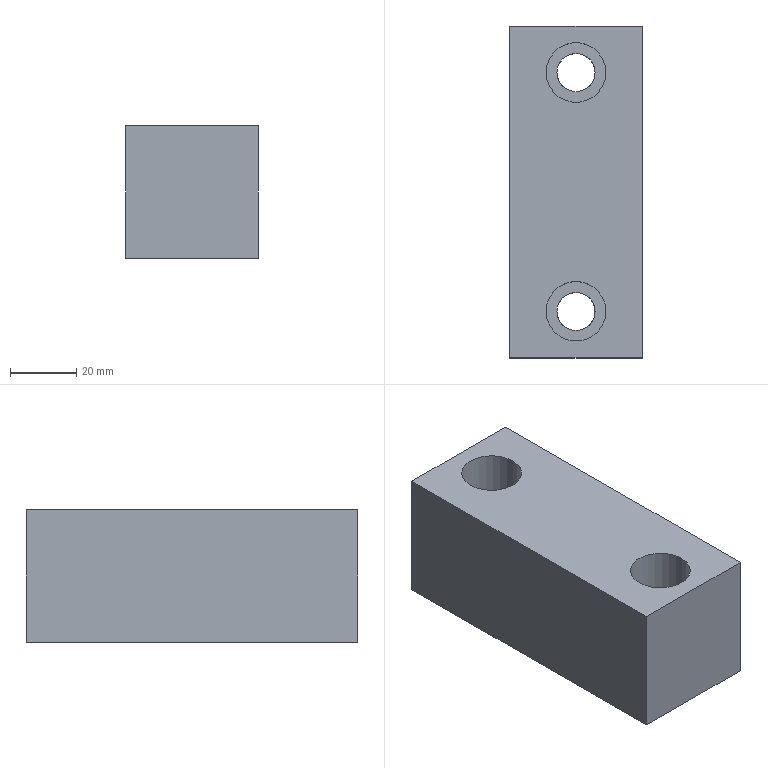Part | STEP file | lll_id4854_x_t | 1 solid | 12 faces | box 40 x 100 x 40 mm | volume 145651 mm3 | plane 8 | cylinder 4 | commonest cylinder face diameters 11.509 x2 18.008 x2
STEP:
#1=CARTESIAN_POINT('',(2439.,39.,-80.));
#2=VERTEX_POINT('',#1);
#3=CARTESIAN_POINT('',(2439.,39.,-40.));
#4=VERTEX_POINT('',#3);
#5=CARTESIAN_POINT('',(2439.,39.,-80.));
#6=DIRECTION('',(0.,0.,1.));
#7=VECTOR('',#6,1.);
#8=LINE('',#5,#7);
#9=EDGE_CURVE('',#2,#4,#8,.T.);
#10=ORIENTED_EDGE('',*,*,#9,.T.);
#11=CARTESIAN_POINT('',(2439.,139.,-40.));
#12=VERTEX_POINT('',#11);
#13=CARTESIAN_POINT('',(2439.,89.,-40.));
#14=DIRECTION('',(0.,1.,0.));
#15=VECTOR('',#14,1.);
#16=LINE('',#13,#15);
#17=EDGE_CURVE('',#4,#12,#16,.T.);
#18=ORIENTED_EDGE('',*,*,#17,.T.);
#19=CARTESIAN_POINT('',(2439.,139.,-80.));
#20=VERTEX_POINT('',#19);
#21=CARTESIAN_POINT('',(2439.,139.,-80.));
#22=DIRECTION('',(0.,0.,1.));
#23=VECTOR('',#22,1.);
#24=LINE('',#21,#23);
#25=EDGE_CURVE('',#20,#12,#24,.T.);
#26=ORIENTED_EDGE('',*,*,#25,.F.);
#27=CARTESIAN_POINT('',(2439.,89.,-80.));
#28=DIRECTION('',(0.,1.,0.));
#29=VECTOR('',#28,1.);
#30=LINE('',#27,#29);
#31=EDGE_CURVE('',#2,#20,#30,.T.);
#32=ORIENTED_EDGE('',*,*,#31,.F.);
#33=EDGE_LOOP('',(#10,#18,#26,#32));
#34=FACE_OUTER_BOUND('',#33,.T.);
#35=CARTESIAN_POINT('',(2439.,89.,-80.));
#36=DIRECTION('',(-1.,0.,0.));
#37=DIRECTION('',(0.,0.,-1.));
#38=AXIS2_PLACEMENT_3D('',#35,#36,#37);
#39=PLANE('',#38);
#40=ADVANCED_FACE('',(#34),#39,.T.);
#41=CARTESIAN_POINT('',(2479.,39.,-80.));
#42=VERTEX_POINT('',#41);
#43=CARTESIAN_POINT('',(2479.,39.,-40.));
#44=VERTEX_POINT('',#43);
#45=CARTESIAN_POINT('',(2479.,39.,-80.));
#46=DIRECTION('',(0.,0.,1.));
#47=VECTOR('',#46,1.);
#48=LINE('',#45,#47);
#49=EDGE_CURVE('',#42,#44,#48,.T.);
#50=ORIENTED_EDGE('',*,*,#49,.T.);
#51=CARTESIAN_POINT('',(2449.,39.,-40.));
#52=DIRECTION('',(-1.,0.,0.));
#53=VECTOR('',#52,1.);
#54=LINE('',#51,#53);
#55=EDGE_CURVE('',#44,#4,#54,.T.);
#56=ORIENTED_EDGE('',*,*,#55,.T.);
#57=ORIENTED_EDGE('',*,*,#9,.F.);
#58=CARTESIAN_POINT('',(2449.,39.,-80.));
#59=DIRECTION('',(-1.,0.,0.));
#60=VECTOR('',#59,1.);
#61=LINE('',#58,#60);
#62=EDGE_CURVE('',#42,#2,#61,.T.);
#63=ORIENTED_EDGE('',*,*,#62,.F.);
#64=EDGE_LOOP('',(#50,#56,#57,#63));
#65=FACE_OUTER_BOUND('',#64,.T.);
#66=CARTESIAN_POINT('',(2449.,39.,-80.));
#67=DIRECTION('',(0.,-1.,0.));
#68=DIRECTION('',(0.,0.,1.));
#69=AXIS2_PLACEMENT_3D('',#66,#67,#68);
#70=PLANE('',#69);
#71=ADVANCED_FACE('',(#65),#70,.T.);
#72=CARTESIAN_POINT('',(2479.,139.,-80.));
#73=VERTEX_POINT('',#72);
#74=CARTESIAN_POINT('',(2479.,139.,-40.));
#75=VERTEX_POINT('',#74);
#76=CARTESIAN_POINT('',(2479.,139.,-80.));
#77=DIRECTION('',(0.,0.,1.));
#78=VECTOR('',#77,1.);
#79=LINE('',#76,#78);
#80=EDGE_CURVE('',#73,#75,#79,.T.);
#81=ORIENTED_EDGE('',*,*,#80,.T.);
#82=CARTESIAN_POINT('',(2479.,89.,-40.));
#83=DIRECTION('',(0.,1.,0.));
#84=VECTOR('',#83,1.);
#85=LINE('',#82,#84);
#86=EDGE_CURVE('',#44,#75,#85,.T.);
#87=ORIENTED_EDGE('',*,*,#86,.F.);
#88=ORIENTED_EDGE('',*,*,#49,.F.);
#89=CARTESIAN_POINT('',(2479.,89.,-80.));
#90=DIRECTION('',(0.,-1.,0.));
#91=VECTOR('',#90,1.);
#92=LINE('',#89,#91);
#93=EDGE_CURVE('',#73,#42,#92,.T.);
#94=ORIENTED_EDGE('',*,*,#93,.F.);
#95=EDGE_LOOP('',(#81,#87,#88,#94));
#96=FACE_OUTER_BOUND('',#95,.T.);
#97=CARTESIAN_POINT('',(2479.,89.,-80.));
#98=DIRECTION('',(1.,0.,0.));
#99=DIRECTION('',(0.,0.,1.));
#100=AXIS2_PLACEMENT_3D('',#97,#98,#99);
#101=PLANE('',#100);
#102=ADVANCED_FACE('',(#96),#101,.T.);
#103=ORIENTED_EDGE('',*,*,#25,.T.);
#104=CARTESIAN_POINT('',(2449.,139.,-40.));
#105=DIRECTION('',(-1.,0.,0.));
#106=VECTOR('',#105,1.);
#107=LINE('',#104,#106);
#108=EDGE_CURVE('',#75,#12,#107,.T.);
#109=ORIENTED_EDGE('',*,*,#108,.F.);
#110=ORIENTED_EDGE('',*,*,#80,.F.);
#111=CARTESIAN_POINT('',(2449.,139.,-80.));
#112=DIRECTION('',(1.,0.,0.));
#113=VECTOR('',#112,1.);
#114=LINE('',#111,#113);
#115=EDGE_CURVE('',#20,#73,#114,.T.);
#116=ORIENTED_EDGE('',*,*,#115,.F.);
#117=EDGE_LOOP('',(#103,#109,#110,#116));
#118=FACE_OUTER_BOUND('',#117,.T.);
#119=CARTESIAN_POINT('',(2449.,139.,-80.));
#120=DIRECTION('',(0.,1.,0.));
#121=DIRECTION('',(0.,0.,-1.));
#122=AXIS2_PLACEMENT_3D('',#119,#120,#121);
#123=PLANE('',#122);
#124=ADVANCED_FACE('',(#118),#123,.T.);
#125=CARTESIAN_POINT('',(2449.996,53.,-60.));
#126=VERTEX_POINT('',#125);
#127=CARTESIAN_POINT('',(2459.,53.,-60.));
#128=DIRECTION('',(0.,0.,1.));
#129=DIRECTION('',(-1.,0.,0.));
#130=AXIS2_PLACEMENT_3D('',#127,#128,#129);
#131=CIRCLE('',#130,9.004);
#132=EDGE_CURVE('',#126,#126,#131,.T.);
#133=ORIENTED_EDGE('',*,*,#132,.F.);
#134=EDGE_LOOP('',(#133));
#135=FACE_BOUND('',#134,.T.);
#136=CARTESIAN_POINT('',(2468.004,53.,-40.));
#137=VERTEX_POINT('',#136);
#138=CARTESIAN_POINT('',(2459.,53.,-40.));
#139=DIRECTION('',(0.,0.,-1.));
#140=DIRECTION('',(1.,0.,0.));
#141=AXIS2_PLACEMENT_3D('',#138,#139,#140);
#142=CIRCLE('',#141,9.004);
#143=EDGE_CURVE('',#137,#137,#142,.T.);
#144=ORIENTED_EDGE('',*,*,#143,.F.);
#145=EDGE_LOOP('',(#144));
#146=FACE_BOUND('',#145,.T.);
#147=CARTESIAN_POINT('',(2459.,53.,-35.));
#148=DIRECTION('',(0.,0.,-1.));
#149=DIRECTION('',(0.,1.,0.));
#150=AXIS2_PLACEMENT_3D('',#147,#148,#149);
#151=CYLINDRICAL_SURFACE('',#150,9.004);
#152=ADVANCED_FACE('',(#135,#146),#151,.F.);
#153=CARTESIAN_POINT('',(2449.996,125.,-60.));
#154=VERTEX_POINT('',#153);
#155=CARTESIAN_POINT('',(2459.,125.,-60.));
#156=DIRECTION('',(0.,0.,1.));
#157=DIRECTION('',(-1.,0.,0.));
#158=AXIS2_PLACEMENT_3D('',#155,#156,#157);
#159=CIRCLE('',#158,9.004);
#160=EDGE_CURVE('',#154,#154,#159,.T.);
#161=ORIENTED_EDGE('',*,*,#160,.F.);
#162=EDGE_LOOP('',(#161));
#163=FACE_BOUND('',#162,.T.);
#164=CARTESIAN_POINT('',(2468.004,125.,-40.));
#165=VERTEX_POINT('',#164);
#166=CARTESIAN_POINT('',(2459.,125.,-40.));
#167=DIRECTION('',(0.,0.,1.));
#168=DIRECTION('',(1.,0.,0.));
#169=AXIS2_PLACEMENT_3D('',#166,#167,#168);
#170=CIRCLE('',#169,9.004);
#171=EDGE_CURVE('',#165,#165,#170,.T.);
#172=ORIENTED_EDGE('',*,*,#171,.T.);
#173=EDGE_LOOP('',(#172));
#174=FACE_BOUND('',#173,.T.);
#175=CARTESIAN_POINT('',(2459.,125.,-35.));
#176=DIRECTION('',(0.,0.,-1.));
#177=DIRECTION('',(0.,1.,0.));
#178=AXIS2_PLACEMENT_3D('',#175,#176,#177);
#179=CYLINDRICAL_SURFACE('',#178,9.004);
#180=ADVANCED_FACE('',(#163,#174),#179,.F.);
#181=CARTESIAN_POINT('',(2459.,119.246,-80.));
#182=VERTEX_POINT('',#181);
#183=CARTESIAN_POINT('',(2459.,125.,-80.));
#184=DIRECTION('',(0.,0.,1.));
#185=DIRECTION('',(0.,-1.,0.));
#186=AXIS2_PLACEMENT_3D('',#183,#184,#185);
#187=CIRCLE('',#186,5.755);
#188=EDGE_CURVE('',#182,#182,#187,.T.);
#189=ORIENTED_EDGE('',*,*,#188,.T.);
#190=EDGE_LOOP('',(#189));
#191=FACE_BOUND('',#190,.T.);
#192=CARTESIAN_POINT('',(2459.,47.246,-80.));
#193=VERTEX_POINT('',#192);
#194=CARTESIAN_POINT('',(2459.,53.,-80.));
#195=DIRECTION('',(0.,0.,1.));
#196=DIRECTION('',(0.,-1.,0.));
#197=AXIS2_PLACEMENT_3D('',#194,#195,#196);
#198=CIRCLE('',#197,5.755);
#199=EDGE_CURVE('',#193,#193,#198,.T.);
#200=ORIENTED_EDGE('',*,*,#199,.T.);
#201=EDGE_LOOP('',(#200));
#202=FACE_BOUND('',#201,.T.);
#203=ORIENTED_EDGE('',*,*,#115,.T.);
#204=ORIENTED_EDGE('',*,*,#93,.T.);
#205=ORIENTED_EDGE('',*,*,#62,.T.);
#206=ORIENTED_EDGE('',*,*,#31,.T.);
#207=EDGE_LOOP('',(#203,#204,#205,#206));
#208=FACE_BOUND('',#207,.T.);
#209=CARTESIAN_POINT('',(2449.,89.,-80.));
#210=DIRECTION('',(0.,0.,-1.));
#211=DIRECTION('',(0.,-1.,0.));
#212=AXIS2_PLACEMENT_3D('',#209,#210,#211);
#213=PLANE('',#212);
#214=ADVANCED_FACE('',(#191,#202,#208),#213,.T.);
#215=ORIENTED_EDGE('',*,*,#199,.F.);
#216=EDGE_LOOP('',(#215));
#217=FACE_BOUND('',#216,.T.);
#218=CARTESIAN_POINT('',(2453.245,53.,-60.));
#219=VERTEX_POINT('',#218);
#220=CARTESIAN_POINT('',(2459.,53.,-60.));
#221=DIRECTION('',(0.,0.,1.));
#222=DIRECTION('',(-1.,0.,0.));
#223=AXIS2_PLACEMENT_3D('',#220,#221,#222);
#224=CIRCLE('',#223,5.755);
#225=EDGE_CURVE('',#219,#219,#224,.T.);
#226=ORIENTED_EDGE('',*,*,#225,.T.);
#227=EDGE_LOOP('',(#226));
#228=FACE_BOUND('',#227,.T.);
#229=CARTESIAN_POINT('',(2459.,53.,-33.));
#230=DIRECTION('',(0.,0.,-1.));
#231=DIRECTION('',(0.,1.,0.));
#232=AXIS2_PLACEMENT_3D('',#229,#230,#231);
#233=CYLINDRICAL_SURFACE('',#232,5.755);
#234=ADVANCED_FACE('',(#217,#228),#233,.F.);
#235=ORIENTED_EDGE('',*,*,#225,.F.);
#236=EDGE_LOOP('',(#235));
#237=FACE_BOUND('',#236,.T.);
#238=ORIENTED_EDGE('',*,*,#132,.T.);
#239=EDGE_LOOP('',(#238));
#240=FACE_BOUND('',#239,.T.);
#241=CARTESIAN_POINT('',(2459.,53.,-60.));
#242=DIRECTION('',(0.,0.,-1.));
#243=DIRECTION('',(0.,-1.,0.));
#244=AXIS2_PLACEMENT_3D('',#241,#242,#243);
#245=PLANE('',#244);
#246=ADVANCED_FACE('',(#237,#240),#245,.F.);
#247=ORIENTED_EDGE('',*,*,#188,.F.);
#248=EDGE_LOOP('',(#247));
#249=FACE_BOUND('',#248,.T.);
#250=CARTESIAN_POINT('',(2453.245,125.,-60.));
#251=VERTEX_POINT('',#250);
#252=CARTESIAN_POINT('',(2459.,125.,-60.));
#253=DIRECTION('',(0.,0.,1.));
#254=DIRECTION('',(-1.,0.,0.));
#255=AXIS2_PLACEMENT_3D('',#252,#253,#254);
#256=CIRCLE('',#255,5.755);
#257=EDGE_CURVE('',#251,#251,#256,.T.);
#258=ORIENTED_EDGE('',*,*,#257,.T.);
#259=EDGE_LOOP('',(#258));
#260=FACE_BOUND('',#259,.T.);
#261=CARTESIAN_POINT('',(2459.,125.,-33.));
#262=DIRECTION('',(0.,0.,-1.));
#263=DIRECTION('',(0.,1.,0.));
#264=AXIS2_PLACEMENT_3D('',#261,#262,#263);
#265=CYLINDRICAL_SURFACE('',#264,5.755);
#266=ADVANCED_FACE('',(#249,#260),#265,.F.);
#267=ORIENTED_EDGE('',*,*,#257,.F.);
#268=EDGE_LOOP('',(#267));
#269=FACE_BOUND('',#268,.T.);
#270=ORIENTED_EDGE('',*,*,#160,.T.);
#271=EDGE_LOOP('',(#270));
#272=FACE_BOUND('',#271,.T.);
#273=CARTESIAN_POINT('',(2459.,125.,-60.));
#274=DIRECTION('',(0.,0.,-1.));
#275=DIRECTION('',(0.,-1.,0.));
#276=AXIS2_PLACEMENT_3D('',#273,#274,#275);
#277=PLANE('',#276);
#278=ADVANCED_FACE('',(#269,#272),#277,.F.);
#279=ORIENTED_EDGE('',*,*,#17,.F.);
#280=ORIENTED_EDGE('',*,*,#55,.F.);
#281=ORIENTED_EDGE('',*,*,#86,.T.);
#282=ORIENTED_EDGE('',*,*,#108,.T.);
#283=EDGE_LOOP('',(#279,#280,#281,#282));
#284=FACE_BOUND('',#283,.T.);
#285=ORIENTED_EDGE('',*,*,#171,.F.);
#286=EDGE_LOOP('',(#285));
#287=FACE_BOUND('',#286,.T.);
#288=ORIENTED_EDGE('',*,*,#143,.T.);
#289=EDGE_LOOP('',(#288));
#290=FACE_BOUND('',#289,.T.);
#291=CARTESIAN_POINT('',(1860.,-180.,-40.));
#292=DIRECTION('',(0.,0.,1.));
#293=DIRECTION('',(1.,0.,0.));
#294=AXIS2_PLACEMENT_3D('',#291,#292,#293);
#295=PLANE('',#294);
#296=ADVANCED_FACE('',(#284,#287,#290),#295,.T.);
#297=CLOSED_SHELL('',(#40,#71,#102,#124,#152,#180,#214,#234,#246,#266,#278,#296));
#298=MANIFOLD_SOLID_BREP('',#297);
#299=(LENGTH_UNIT()NAMED_UNIT(*)SI_UNIT(.MILLI.,.METRE.));
#300=UNCERTAINTY_MEASURE_WITH_UNIT(LENGTH_MEASURE(0.00002),#299,'','');
#301=(NAMED_UNIT(*)PLANE_ANGLE_UNIT()SI_UNIT($,.RADIAN.));
#302=PLANE_ANGLE_MEASURE_WITH_UNIT(PLANE_ANGLE_MEASURE(0.01745),#301);
#303=DIMENSIONAL_EXPONENTS(0.,0.,0.,0.,0.,0.,0.);
#304=(CONVERSION_BASED_UNIT('DEGREE',#302)NAMED_UNIT(#303)PLANE_ANGLE_UNIT());
#305=(NAMED_UNIT(*)SI_UNIT($,.STERADIAN.)SOLID_ANGLE_UNIT());
#306=(GEOMETRIC_REPRESENTATION_CONTEXT(3)GLOBAL_UNCERTAINTY_ASSIGNED_CONTEXT((#300))GLOBAL_UNIT_ASSIGNED_CONTEXT((#299,#304,#305))REPRESENTATION_CONTEXT('',''));
#307=ADVANCED_BREP_SHAPE_REPRESENTATION('',(#298),#306);